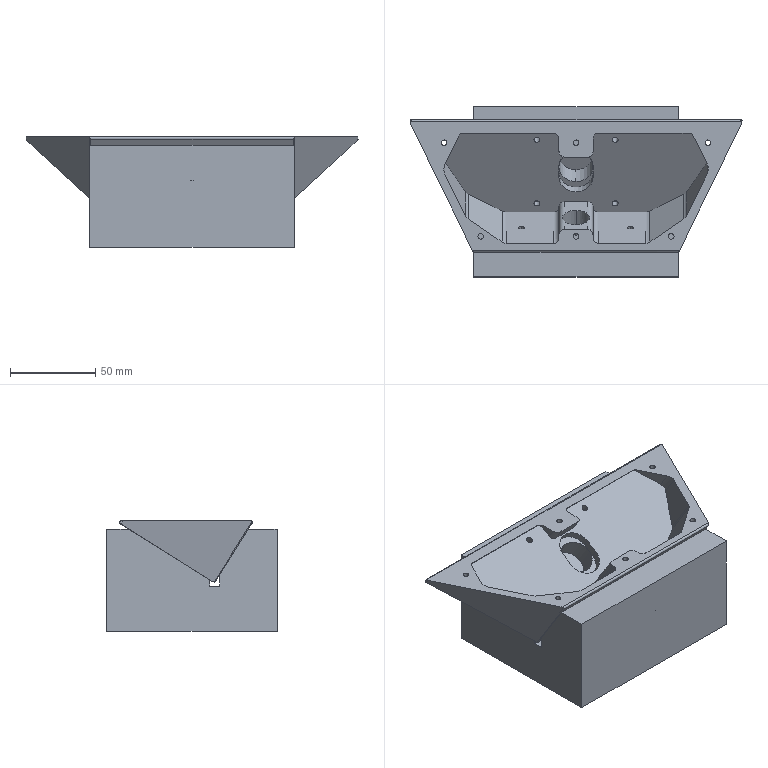NC program | Mastercam | posted with a generic post | part box 195.124 x 100 x 65 mm
Lines 4165 to 4842 of 16336:
N1960 T8 M6
N1970 G0 G90 G17 G57 X-110.144 Y-96.37 A180. S5000 M3
N1980 G43 H8 Z50.
N1990 Z2.
N2000 G1 Z-30.75 F2000.
N2010 X-110.64 Y-95.137 Z-30.87 F4000.
N2020 G3 X-111.435 Y-93.935 Z-31. I-3.34 J-1.343
N2030 G2 X-112.273 Y-92.613 I16.01 J11.086
N2040 X-113.576 Y-88.83 I10.355 J5.683
N2050 X-113.883 Y-85.344 I23.54 J3.826
N2060 X-113.915 Y-81.077 I288.279 J4.267
N2070 X-113.901 Y-78.302 I288.311 J0.
N2080 G1 X-113.898 Y-77.731
N2090 X-113.64 Y-20.441
N2100 X-113.403 Y34.823
N2110 X-113.4 Y84.273
N2120 G2 X-113.401 Y84.454 I13.293 J.181
N2130 X-113.267 Y86.34 I13.294 J0.
N2140 X-111.462 Y90.495 I8.753 J-1.333
N2150 X-108.281 Y93.241 I8.647 J-6.8
N2160 X-105.056 Y94.63 I7.461 J-12.884
N2170 X-101.144 Y95.433 I6.609 J-22.262
N2180 X-95.877 Y95.796 I6.569 J-56.933
N2190 X-86.969 Y95.897 I8.908 J-394.638
N2200 X-85.791 Y95.895 I0. J-394.739
N2210 G1 X-85.208 Y95.896
N2220 X-27.018 Y95.9
N2230 X31.163
N2240 X89.343
N2250 X102.279 Y95.896
N2260 G2 X105.296 Y95.418 I-.106 J-10.441
N2270 X108.627 Y93.428 I-3.009 J-8.816
N2280 X111.314 Y89.692 I-8.103 J-8.664
N2290 X112.58 Y85.789 I-15.667 J-7.237
N2300 X113.189 Y80.814 I-33.929 J-6.676
N2310 X113.376 Y73.478 I-148.458 J-7.468
N2320 X113.395 Y68.203 I-935.543 J-6.004
N2330 G1 X113.396 Y67.62
N2340 X113.4 Y9.431
N2350 Y-48.75
N2360 Y-84.241
N2370 G2 X113.401 Y-84.435 I-13.634 J-.194
N2380 X113.277 Y-86.274 I-13.635 J0.
N2390 X111.503 Y-90.442 I-8.743 J1.26
N2400 X108.331 Y-93.212 I-8.656 J6.71
N2410 X105.1 Y-94.617 I-7.482 J12.788
N2420 X101.182 Y-95.429 I-6.623 J22.106
N2430 X95.91 Y-95.795 I-6.576 J56.467
N2440 X86.999 Y-95.897 I-8.911 J391.025
N2450 X85.822 Y-95.895 I0. J391.127
N2460 G1 X85.238 Y-95.896
N2470 X27.049 Y-95.9
N2480 X-31.132
N2490 X-89.313
N2500 X-102.232 Y-95.897
N2510 G2 X-107.155 Y-94.326 I.188 J9.093
N2520 X-110.442 Y-90.83 I6.221 J9.142
N2530 X-112.018 Y-87.165 I13.024 J7.771
N2540 X-112.848 Y-82.575 I24.925 J6.877
N2550 X-113.124 Y-76.806 I71.423 J6.315
N2560 X-113.155 Y-69.702 I814.918 J7.104
N2570 X-113.135 Y-63.868 I814.949 J0.
N2580 G1 X-113.132 Y-63.286
N2590 X-112.87 Y-5.103
N2600 X-112.704 Y35.018
N2610 X-112.687 Y82.362
N2620 G2 X-109.5 Y89.877 I11.19 J-.312
N2630 X-105.234 Y92.857 I9.984 J-9.751
N2640 X-100.796 Y94.274 I8.212 J-18.06
N2650 X-95.264 Y94.953 I7.658 J-39.495
N2660 X-87.342 Y95.17 I8.137 J-152.602
N2670 X-80.896 Y95.195 I6.996 J-975.226
N2680 G1 X-80.313 Y95.196
N2690 X-22.124 Y95.2
N2700 X36.057
N2710 X94.238
N2720 X99.599 Y95.194
N2730 G2 X107.56 Y91.821 I-.061 J-11.226
N2740 X110.444 Y87.541 I-10.109 J-9.924
N2750 X111.729 Y83.509 I-18.496 J-8.115
N2760 X112.396 Y78.597 I-35.731 J-7.351
N2770 X112.657 Y71.195 I-121.795 J-7.996
N2780 X112.697 Y62.365 I-967.338 J-8.83
N2790 G1 Y61.813
N2800 Y61.23
N2810 X112.7 Y3.044
N2820 Y-55.137
N2830 X112.696 Y-81.997
N2840 Y-82.038
N2850 G2 X109.422 Y-89.958 I-11.218 J0.
N2860 X105.15 Y-92.895 I-9.965 J9.918
N2870 X100.721 Y-94.289 I-8.18 J18.255
N2880 X95.2 Y-94.957 I-7.639 J39.98
N2890 X87.283 Y-95.171 I-8.129 J154.832
N2900 X80.838 Y-95.195 I-6.994 J990.575
N2910 G1 X80.255 Y-95.196
N2920 X22.066 Y-95.2
N2930 X-36.115
N2940 X-94.295
N2950 G2 X-95.459 Y-95.201 I-1.164 J858.632
N2960 X-99.439 Y-95.192 I0. J858.633
N2970 X-107.347 Y-91.783 I.221 J11.391
N2980 X-110.234 Y-87.511 I10.125 J9.954
N2990 X-111.605 Y-83.086 I18.397 J8.125
N3000 X-112.252 Y-77.562 I39.964 J7.481
N3010 X-112.433 Y-70.113 I153.565 J7.449
N3020 X-112.432 Y-69.642 I153.746 J0.
N3030 X-112.435 Y-67.053 I976.965 J2.589
N3040 X-112.428 Y-63.196 I976.968 J0.
N3050 G1 X-112.426 Y-62.613
N3060 X-112.167 Y-4.424
N3070 X-112.007 Y34.536
N3080 X-111.994 Y79.432
N3090 G2 X-111.614 Y82.796 I15.366 J-.035
N3100 X-107.699 Y89.359 I12.416 J-2.956
N3110 X-103.194 Y92.184 I10.539 J-11.805
N3120 X-98.579 Y93.554 I8.897 J-21.507
N3130 X-93.139 Y94.214 I8.032 J-43.464
N3140 X-85.207 Y94.459 I8.497 J-146.591
N3150 X-77. Y94.495 I8.38 J-972.399
N3160 G1 X-76.417 Y94.496
N3170 X-18.229 Y94.5
N3180 X39.952
N3190 X97.12 Y94.491
N3200 G2 X100.557 Y94.049 I-.153 J-14.801
N3210 X107.028 Y90.01 I-3.245 J-12.399
N3220 X109.593 Y85.905 I-12.013 J-10.362
N3230 X111.016 Y81.27 I-20.967 J-8.975
N3240 X111.703 Y75.808 I-42.228 J-8.079
N3250 X111.957 Y67.862 I-141.645 J-8.518
N3260 X111.995 Y59.239 I-971.133 J-8.623
N3270 X111.996 Y59.07 I-971.171 J0.
N3280 G1 Y58.487
N3290 X112. Y.3
N3300 Y-57.881
N3310 X111.992 Y-79.538
N3320 G2 X111.578 Y-82.945 I-15.031 J.101
N3330 X107.591 Y-89.456 I-12.407 J3.12
N3340 X103.493 Y-92.054 I-10.412 J11.892
N3350 X98.849 Y-93.5 I-9.007 J20.745
N3360 X93.377 Y-94.198 I-8.1 J41.734
N3370 X85.425 Y-94.457 I-8.527 J139.687
N3380 X76.801 Y-94.496 I-8.624 J956.163
N3390 G1 X76.632
N3400 X76.049
N3410 X17.862 Y-94.5
N3420 X-40.319
N3430 X-96.941 Y-94.488
N3440 G2 X-100.372 Y-94.027 I.247 J14.859
N3450 X-106.816 Y-89.989 I3.313 J12.447
N3460 X-109.383 Y-85.887 I12.018 J10.375
N3470 X-110.808 Y-81.242 I20.845 J8.937
N3480 X-111.484 Y-75.766 I41.728 J7.934
N3490 X-111.709 Y-67.852 I138.785 J7.914
N3500 X-111.71 Y-67.812 I139.01 J0.
N3510 X-111.72 Y-63.445 I943.857 J4.367
N3520 X-111.709 Y-59.017 I943.867 J0.
N3530 G1 X-111.707 Y-58.435
N3540 X-111.448 Y-.247
N3550 X-111.308 Y34.64
N3560 X-111.29 Y77.225
N3570 G2 X-110.964 Y80.662 I19.033 J-.074
N3580 X-105.882 Y88.956 I13.626 J-2.645
N3590 X-101.909 Y91.299 I10.628 J-13.476
N3600 X-96.649 Y92.842 I9.539 J-22.781
N3610 X-90.639 Y93.525 I8.512 J-48.125
N3620 X-82.156 Y93.762 I9.137 J-175.663
N3630 X-75.124 Y93.793 I7.919 J-979.259
N3640 G1 X-74.541 Y93.794
N3650 X-16.35 Y93.8
N3660 X41.831
N3670 X94.251 Y93.796
N3680 X94.346
N3690 G2 X97.476 Y93.582 I0. J-23.005
N3700 X106.327 Y88.541 I-1.957 J-13.725
N3710 X108.727 Y84.575 I-13.198 J-10.696
N3720 X110.314 Y79.299 I-22.353 J-9.599
N3730 X111.017 Y73.273 I-47.106 J-8.549
N3740 X111.26 Y64.781 I-171.165 J-9.153
N3750 X111.294 Y57.163 I-987.039 J-8.154
N3760 G1 X111.295 Y56.58
N3770 X111.3 Y-1.61
N3780 Y-59.791
N3790 X111.286 Y-77.4
N3800 G2 X110.914 Y-80.902 I-18.234 J.166
N3810 X106.081 Y-88.794 I-13.556 J2.876
N3820 X102.116 Y-91.209 I-10.714 J13.128
N3830 X96.835 Y-92.807 I-9.614 J22.247
N3840 X90.803 Y-93.515 I-8.559 J46.873
N3850 X82.309 Y-93.76 I-9.156 J170.159
N3860 X74.691 Y-93.794 I-8.155 J980.687
N3870 G1 X74.108 Y-93.795
N3880 X15.918 Y-93.8
N3890 X-42.263
N3900 X-94.119 Y-93.794
N3910 X-94.141
N3920 G2 X-97.383 Y-93.556 I0. J22.159
N3930 X-106.18 Y-88.448 I2.103 J13.749
N3940 X-108.554 Y-84.474 I13.317 J10.652
N3950 X-110.115 Y-79.194 I22.463 J9.515
N3960 X-110.793 Y-73.164 I47.16 J8.353
N3970 X-110.999 Y-64.77 I170.528 J8.394
N3980 G1 Y-64.67
N3990 G2 X-111.006 Y-60.93 I978.29 J3.74
N4000 X-110.999 Y-57.052 I978.297 J0.
N4010 G1 X-110.997 Y-56.468
N4020 X-110.739 Y1.721
N4030 X-110.609 Y34.863
N4040 X-110.588 Y75.112
N4050 G2 X-110.308 Y78.659 I24.803 J-.171
N4060 X-104.495 Y88.27 I14.593 J-2.263
N4070 X-99.855 Y90.797 I11.125 J-14.904
N4080 X-94.728 Y92.165 I9.618 J-25.766
N4090 X-88.161 Y92.847 I9.097 J-55.599
N4100 X-79.133 Y93.066 I9.529 J-206.878
N4110 X-73.86 Y93.09 I7.037 J-961.297
N4120 G1 X-73.276 Y93.091
N4130 X-15.081 Y93.1
N4140 X43.1
N4150 X92.026 Y93.095
N4160 X92.103
N4170 G2 X95.789 Y92.865 I0. J-29.661
N4180 X102.272 Y90.377 I-1.973 J-14.827
N4190 X106.615 Y85.767 I-8.836 J-12.674
N4200 X108.718 Y81.155 I-17.073 J-10.572
N4210 X109.932 Y75.456 I-31.105 J-9.607
N4220 X110.443 Y68.451 I-74.269 J-8.933
N4230 X110.589 Y57.784 I-389.902 J-10.667
N4240 X110.588 Y57.188 I-390.048 J0.
N4250 G1 X110.59 Y56.604
N4260 X110.6 Y-1.594
N4270 Y-45.803
N4280 G3 X110.619 Y-46.052 I1.6 J0.
N4290 G2 X110.718 Y-47.313 I-8.001 J-1.261
N4300 X110.704 Y-47.792 I-8.1 J0.
N4310 G3 X110.603 Y-56.28 I357.176 J-8.488
N4320 X110.605 Y-57.469 I357.277 J0.
N4330 G1 X110.604 Y-58.049
N4340 X110.589 Y-75.017
N4350 G2 X110.33 Y-78.525 I-25.607 J.131
N4360 X104.608 Y-88.185 I-14.604 J2.126
N4370 X99.97 Y-90.753 I-11.173 J14.703
N4380 X94.833 Y-92.146 I-9.656 J25.437
N4390 X88.882 Y-92.806 I-8.741 J51.682
N4400 X80.401 Y-93.054 I-9.378 J175.223
N4410 X72.196 Y-93.093 I-8.788 J988.587
N4420 G1 X71.613 Y-93.094
N4430 X13.423 Y-93.1
N4440 X-44.758
N4450 X-91.959 Y-93.093
N4460 X-92.108
N4470 G2 X-95.798 Y-92.826 I0. J25.572
N4480 X-105.74 Y-86.737 I2.149 J14.671
N4490 X-108.033 Y-82.473 I15.2 J10.92
N4500 X-109.424 Y-77.325 I25.264 J9.589
N4510 X-110.069 Y-71.363 I51.092 J8.544
N4520 X-110.285 Y-62.875 I172.118 J8.62
N4530 X-110.295 Y-58.357 I998.404 J4.518
N4540 X-110.286 Y-54.086 I998.414 J0.
N4550 G1 X-110.284 Y-53.503
N4560 X-110.272 Y-50.228
N4570 Y-50.221
N4580 G3 X-110.345 Y-49.742 I-1.6 J0.
N4590 G2 X-110.718 Y-47.313 I7.727 J2.429
N4600 X-110.617 Y-46.038 I8.1 J0.
N4610 G3 X-110.334 Y-42.078 I-42.325 J5.013
N4620 X-110.198 Y-32.387 I-384.119 J10.238
N4630 G1 X-110.195 Y-31.807
N4640 X-109.931 Y26.358
N4650 X-109.9 Y54.843
N4660 X-109.889 Y72.971
N4670 G2 X-109.661 Y76.644 I32.598 J-.178
N4680 X-108.002 Y82.061 I16.294 J-2.028
N4690 X-103.238 Y87.548 I13.99 J-7.335
N4700 X-98.687 Y89.986 I11.398 J-15.815
N4710 X-92.914 Y91.49 I10.304 J-27.707
N4720 X-86.407 Y92.138 I9.263 J-60.01
N4730 X-76.798 Y92.366 I10.148 J-225.103
N4740 X-72.112 Y92.388 I6.994 J-991.545
N4750 G1 X-71.528 Y92.39
N4760 X-13.331 Y92.4
N4770 X44.85
N4780 X90.309 Y92.391
N4790 G2 X93.93 Y92.189 I-.128 J-34.771
N4800 X99.337 Y90.616 I-1.871 J-16.513
N4810 X105.181 Y85.553 I-7.137 J-14.143
N4820 X107.692 Y80.629 I-16.412 J-11.47
N4830 X109.07 Y74.905 I-29.456 J-10.122
N4840 X109.662 Y68.446 I-64.438 J-9.157
N4850 X109.873 Y58.273 I-252.428 J-10.337
N4860 X109.884 Y55.93 I-975.06 J-5.747
N4870 G1 X109.886 Y55.345
N4880 X109.9 Y-2.857
N4890 X109.904 Y-43.436
N4900 G3 X110.038 Y-44.065 I1.6 J.013
N4910 G2 X110.718 Y-47.313 I-7.42 J-3.248
N4920 X110.498 Y-49.19 I-8.1 J0.
N4930 G3 X110.159 Y-51.609 I17.042 J-3.62
N4940 X109.951 Y-56.961 I84.4 J-5.966
N4950 X109.901 Y-66.881 I979.191 J-9.92
N4960 X109.902 Y-68.499 I979.241 J0.
N4970 G1 X109.901 Y-69.08
N4980 G2 X109.904 Y-70.102 I-204.889 J-1.022
N4990 X109.868 Y-73.943 I-204.892 J0.
N5000 X109.447 Y-77.921 I-23.081 J.43
N5010 X103.258 Y-87.534 I-15.216 J2.998
N5020 X98.707 Y-89.978 I-11.406 J15.779
N5030 X92.932 Y-91.487 I-10.31 J27.645
N5040 X86.424 Y-92.137 I-9.267 J59.859
N5050 X76.814 Y-92.366 I-10.15 J224.438
N5060 X72.127 Y-92.388 I-6.994 J988.318
N5070 G1 X71.543 Y-92.39
N5080 X13.346 Y-92.4
N5090 X-44.835
N5100 X-90.317 Y-92.387
N5110 G2 X-94.01 Y-92.146 I.211 J31.66
N5120 X-99.862 Y-90.216 I2.05 J16.051
N5130 X-105.145 Y-85.288 I7.987 J13.857
N5140 X-107.564 Y-80.355 I16.841 J11.322
N5150 X-108.877 Y-74.644 I30.151 J9.939
N5160 X-109.423 Y-68.196 I66.024 J8.837
N5170 X-109.585 Y-59.036 I258.916 J9.16
N5180 X-109.583 Y-58.03 I259.078 J0.
N5190 X-109.584 Y-56.798 I999.64 J1.232
N5200 X-109.583 Y-55.687 I999.641 J0.
N5210 G1 Y-55.102
N5220 G3 X-109.577 Y-54.037 I-96.819 J1.065
N5230 X-109.6 Y-51.939 I-96.825 J0.
N5240 G1 Y-51.898
N5250 G3 X-109.756 Y-51.173 I-1.745 J0.
N5260 G2 X-110.384 Y-49.616 I8.804 J4.451
N5270 G3 X-111.062 Y-48.344 Z-30.928 I-3.451 J-1.024
N5280 G1 X-111.872 Y-47.366 Z-30.865
N5290 G3 X-113.723 Y-46.035 Z-30.75 I-3.47 J-2.872
N5300 X-115.342 Y-45.734 I-1.619 J-4.203 F9500.
N5310 X-119.846 Y-50.238 I0. J-4.504
N5320 X-119.607 Y-51.684 I4.504 J0.
N5330 G1 X-108.76 Y-83.666
N5340 G3 X-95.326 Y-93.494 I13.715 J4.652
N5350 G1 X75.09 Y-96.795
N5360 G3 X76.259 Y-96.806 I1.169 J60.307
N5370 X103.006 Y-90.552 I0. J60.318
N5380 X110.559 Y-81.171 I-6.356 J12.848
N5390 G1 X118.041 Y-51.155
N5400 G3 X118.47 Y-47.625 I-14.298 J3.53
N5410 X118.467 Y-47.295 I-14.727 J0.
N5420 X114.973 Y-43.801 I-3.494 J0.
N5430 X113.316 Y-44.219 I0. J-3.494
N5440 X111.957 Y-45.531 Z-30.845 I1.657 J-3.076 F4000.
N5450 G1 X111.759 Y-45.87 Z-30.865
N5460 X111.118 Y-46.967 Z-30.928
N5470 G3 X110.654 Y-48.332 Z-31. I3.107 J-1.817
N5480 G2 X110.148 Y-50.298 I-8.036 J1.019
N5490 G3 X109.688 Y-52.399 I11.349 J-3.588
N5500 X109.339 Y-56.906 I43.841 J-5.657
N5510 X109.209 Y-65.826 I306.543 J-8.92
N5520 X109.21 Y-66.56 I306.673 J0.
N5530 G1 X109.209 Y-67.139
N5540 G2 X109.21 Y-67.831 I-199.938 J-.692
N5550 X109.152 Y-72.626 I-199.939 J0.
N5560 X108.643 Y-76.934 I-24.188 J.674
N5570 X102.242 Y-86.685 I-15.76 J3.37
N5580 X97.024 Y-89.391 I-11.998 J16.749
N5590 X91.334 Y-90.793 I-10.402 J29.975
N5600 X84.865 Y-91.425 I-9.439 J63.161
N5610 X75.257 Y-91.662 I-10.335 J224.793
N5620 X69.984 Y-91.688 I-7.391 J961.364
N5630 G1 X69.4 Y-91.689
N5640 X11.203 Y-91.7
N5650 X-46.977
N5660 X-88.376 Y-91.687
N5670 G2 X-92.672 Y-91.416 I.047 J34.843
N5680 X-97.486 Y-90.063 I2.284 J17.373
N5690 X-104.052 Y-84.618 I6.752 J14.822
N5700 X-106.714 Y-79.388 I16.859 J11.873
N5710 X-108.079 Y-73.698 I30.219 J10.257
N5720 X-108.678 Y-67.231 I63.598 J9.151
N5730 X-108.87 Y-57.914 I226.012 J9.317
N5740 X-108.869 Y-57.624 I226.204 J0.
N5750 X-108.874 Y-55.871 I902.406 J3.145
N5760 G3 X-108.87 Y-55.345 I-32.379 J.526
N5770 X-108.946 Y-53.127 I-32.383 J0.
N5780 X-109.099 Y-52.56 I-1.595 J-.128
N5790 G2 X-109.974 Y-50.704 I109.099 J52.56
N5800 G3 X-110.827 Y-49.543 Z-30.928 I-3.269 J-1.508
N5810 G1 X-111.769 Y-48.69 Z-30.865
N5820 G3 X-113.801 Y-47.661 Z-30.75 I-2.898 J-3.201
N5830 X-114.667 Y-47.573 I-.866 J-4.23 F9500.
N5840 X-118.985 Y-51.891 I0. J-4.318
N5850 X-118.721 Y-53.377 I4.318 J0.
N5860 G1 X-108.315 Y-81.777
N5870 G3 X-90.706 Y-94.115 I17.662 J6.472
N5880 G1 X86.503 Y-94.617
N5890 X86.579
N5900 G3 X109.028 Y-82.514 I0. J26.872
N5910 X110.11 Y-80.135 I-7.069 J4.651
N5920 G1 X118.414 Y-50.339
N5930 G3 X118.552 Y-49.33 I-3.62 J1.009
N5940 X116.178 Y-45.837 I-3.758 J0.
N5950 X114.867 Y-45.587 I-1.311 J-3.309
N5960 X113.66 Y-45.798 I0. J-3.559
N5970 X112.083 Y-46.928 Z-30.848 I1.207 J-3.348 F4000.
N5980 G1 X111.871 Y-47.194 Z-30.865
N5990 X111.08 Y-48.187 Z-30.928
N6000 G3 X110.425 Y-49.471 Z-31. I2.815 J-2.244
N6010 G2 X109.729 Y-51.232 I-9.276 J2.649
N6020 G3 X109.189 Y-53.22 I9.872 J-3.751
N6030 X108.726 Y-57.554 I34.204 J-5.841
N6040 X108.532 Y-65.368 I173.33 J-8.223
N6050 X108.52 Y-67.102 I929.99 J-7.448
N6060 G2 X108.521 Y-67.431 I-89.043 J-.329
N6070 X108.395 Y-72.162 I-89.044 J0.
N6080 X107.701 Y-76.556 I-22.598 J1.313
N6090 X101.459 Y-85.706 I-16.084 J4.27
N6100 X96.684 Y-88.329 I-12.183 J16.515
N6110 X90.972 Y-89.907 I-10.883 J28.275
N6120 X84.441 Y-90.653 I-9.841 J57.18
N6130 X75.37 Y-90.941 I-10.21 J178.514
N6140 X65.993 Y-90.992 I-9.954 J974.623
N6150 G1 X65.409 Y-90.993
N6160 X7.218 Y-91.
N6170 X-50.963
N6180 X-86.534 Y-90.987
N6190 G2 X-90.654 Y-90.781 I.107 J43.297
N6200 X-95.271 Y-89.744 I1.903 J19.263
N6210 X-103.064 Y-83.848 I5.71 J15.645
N6220 X-105.65 Y-79.06 I16.66 J12.092
N6230 X-107.191 Y-73.345 I28.477 J10.746
N6240 X-107.904 Y-66.815 I57.53 J9.579
N6250 X-108.151 Y-57.763 I181.345 J9.481
N6260 G1 Y-57.644
N6270 G3 X-108.237 Y-54.769 I-47.826 J0.
N6280 G1 Y-54.76
N6290 G3 X-108.422 Y-53.942 I-1.895 J0.
N6300 G2 X-109.439 Y-51.849 I108.422 J53.942
N6310 G3 X-110.304 Y-50.696 Z-30.928 I-3.253 J-1.541
N6320 G1 X-111.598 Y-49.55 Z-30.842
N6330 G3 X-113.196 Y-48.653 Z-30.75 I-2.862 J-3.229
N6340 X-114.46 Y-48.464 I-1.264 J-4.126 F9500.
N6350 X-118.775 Y-52.779 I0. J-4.315
N6360 X-118.446 Y-54.434 I4.315 J0.
N6370 G1 X-107.217 Y-81.469
N6380 G3 X-89.476 Y-93.311 I17.741 J7.368
N6390 X-89.409 Y-93.312 I0. J19.21
N6400 G1 X86.808 Y-92.7
N6410 G3 X106.398 Y-84.378 I-.095 J27.444
N6420 X108.723 Y-80.838 I-8.047 J7.817
N6430 G1 X119.405 Y-54.934
N6440 G3 X119.82 Y-52.838 I-5.082 J2.096
N6450 X114.323 Y-47.341 I-5.497 J0.
N6460 X113.852 Y-47.372 I0. J-3.6
N6470 X111.813 Y-48.361 Z-30.865 I.471 J-3.569 F4000.
N6480 G1 X110.902 Y-49.246 Z-30.928
N6490 G3 X110.091 Y-50.438 Z-31. I2.51 J-2.581
N6500 G2 X109.232 Y-52.284 I-66.541 J29.848
N6510 G3 X108.563 Y-54.604 I9.661 J-4.041
N6520 X108.07 Y-58.945 I34.652 J-6.137
N6530 X107.846 Y-66.178 I149.823 J-8.252
N6540 G2 X107.711 Y-70.583 I-98.785 J.832
N6550 X107.017 Y-75.222 I-25.108 J1.386
N6560 X100.399 Y-84.963 I-16.635 J4.182
N6570 X95.313 Y-87.68 I-12.54 J17.358
N6580 X89.654 Y-89.195 I-10.998 J29.743
N6590 X83.147 Y-89.936 I-10.009 J58.979
N6600 X74.076 Y-90.235 I-10.386 J177.553
N6610 X64.11 Y-90.291 I-10.34 J941.175
N6620 G1 X63.527 Y-90.292
N6630 X5.335 Y-90.3
N6640 X-52.846
N6650 X-84.925 Y-90.286
N6660 G2 X-89.711 Y-90.024 I.12 J46.114
N6670 X-94.684 Y-88.798 I2.149 J19.409
N6680 X-102.271 Y-82.852 I6.366 J15.936
N6690 X-104.971 Y-77.753 I17.383 J12.469
N6700 X-106.464 Y-72.087 I29.755 J10.873
N6710 X-107.178 Y-65.576 I58.911 J9.752
N6720 X-107.427 Y-58.363 I181.424 J9.883
N6730 G3 X-107.562 Y-55.865 I-27.085 J-.212
N6740 X-107.729 Y-55.315 I-1.59 J-.181
N6750 G2 X-108.772 Y-53.235 I107.729 J55.315
N6760 G3 X-109.652 Y-52.093 Z-30.928 I-3.233 J-1.582
N6770 G1 X-111.212 Y-50.744 Z-30.825
N6780 G3 X-112.503 Y-49.969 Z-30.75 I-2.887 J-3.342
N6790 X-114.099 Y-49.67 I-1.596 J-4.117 F9500.
N6800 X-118.515 Y-54.086 I0. J-4.416
N6810 X-118.083 Y-55.99 I4.416 J0.
N6820 G1 X-105.653 Y-81.998
N6830 G3 X-88.458 Y-92.838 I17.195 J8.218
N6840 G1 X-88.343
N6850 X86.078 Y-91.792
N6860 G3 X105.628 Y-83.346 I-.163 J27.226
N6870 X107.415 Y-80.743 I-7.193 J6.853
N6880 G1 X119.173 Y-55.895
N6890 G3 X119.69 Y-53.595 I-4.861 J2.3
N6900 X114.312 Y-48.217 I-5.378 J0.
N6910 X113.338 Y-48.305 I0. J-5.378
N6920 X113.073 Y-48.36 Z-30.763 I.974 J-5.29 F4000.
N6930 X112.142 Y-48.846 Z-30.816 I.492 J-2.08
N6940 G1 X111.662 Y-49.274 Z-30.848
N6950 X110.467 Y-50.34 Z-30.928
N6960 G3 X109.606 Y-51.495 Z-31. I2.397 J-2.686
N6970 G2 X108.575 Y-53.656 I-109.911 J51.125
N6980 G3 X107.891 Y-56.116 I11.101 J-4.409
N6990 X107.393 Y-60.503 I36.793 J-6.404
N7000 X107.152 Y-66.68 I170.39 J-9.732
N7010 G2 X106.815 Y-71.398 I-49.471 J1.157
N7020 X105.602 Y-76.255 I-20.844 J2.628
N7030 X99.527 Y-84.111 I-16.428 J6.426
N7040 X94.486 Y-86.839 I-12.771 J17.579
N7050 X88.839 Y-88.403 I-11.261 J29.681
N7060 X81.693 Y-89.234 I-10.463 J58.847
N7070 X72.041 Y-89.539 I-10.934 J193.463
N7080 X62.665 Y-89.59 I-10.219 J999.503
N7090 G1 X62.082 Y-89.592
N7100 X3.889 Y-89.6
N7110 X-54.292
N7120 X-82.858 Y-89.59
N7130 G2 X-87.444 Y-89.415 I.089 J62.785
N7140 X-92.161 Y-88.556 I1.827 J23.409
N7150 X-101.343 Y-82.077 I4.983 J16.807
N7160 X-104.087 Y-77.027 I17.41 J12.733
N7170 X-105.651 Y-71.369 I29.386 J11.165
N7180 X-106.424 Y-64.837 I56.832 J10.039
N7190 X-106.704 Y-58.914 I194.477 J12.172
N7200 G3 X-106.838 Y-57.247 I-20.355 J-.789
N7210 X-107.013 Y-56.688 I-1.588 J-.19
N7220 G2 X-108.082 Y-54.621 I107.013 J56.688
N7230 G3 X-108.976 Y-53.491 Z-30.928 I-3.213 J-1.624
N7240 G1 X-110.576 Y-52.145 Z-30.824
N7250 G3 X-111.859 Y-51.414 Z-30.75 I-2.618 J-3.11
N7260 X-113.194 Y-51.189 I-1.335 J-3.841 F9500.
N7270 X-117.26 Y-55.255 I0. J-4.066
N7280 X-116.821 Y-57.094 I4.066 J0.
N7290 G1 X-103.744 Y-82.884
N7300 G3 X-87.579 Y-92.812 I16.165 J8.196
N7310 G1 X-87.544
N7320 X84.208 Y-92.481
N7330 G3 X107.762 Y-77.23 I-.05 J25.892
N7340 G1 X117.835 Y-54.883
N7350 G3 X118.194 Y-53.215 I-3.701 J1.668
N7360 X114.134 Y-49.155 I-4.06 J0.
N7370 X112.791 Y-49.384 I0. J-4.06
N7380 X111.463 Y-50.157 Z-30.827 I1.343 J-3.831 F4000.
N7390 G1 X111.409 Y-50.205 Z-30.83
N7400 X109.935 Y-51.493 Z-30.928
N7410 G3 X109.061 Y-52.639 Z-31. I2.368 J-2.711
N7420 G2 X108.05 Y-54.685 I-109.061 J52.639
N7430 G3 X107.328 Y-56.999 I9.625 J-4.274
N7440 X106.762 Y-61.289 I32.504 J-6.469
N7450 X106.476 Y-66.361 I187.201 J-13.099
N7460 G2 X105.981 Y-71.183 I-42.427 J1.917
N7470 X104.356 Y-76.426 I-19.835 J3.276
N7480 X99.326 Y-82.768 I-16.298 J7.76
N7490 X93.644 Y-86.019 I-13.512 J17.025
N7500 X87.336 Y-87.745 I-11.678 J30.28
N7510 X80.234 Y-88.536 I-10.546 J62.439
N7520 X70.594 Y-88.836 I-11.057 J200.229
N7530 X61.218 Y-88.89 I-10.345 J991.635
N7540 G1 X60.635 Y-88.891
N7550 X2.442 Y-88.9
N7560 X-55.739
N7570 X-81.399 Y-88.888
N7580 X-81.477
N7590 G2 X-86.647 Y-88.664 I0. J59.71
N7600 X-91.347 Y-87.743 I2.151 J23.445
N7610 X-100.154 Y-81.669 I5.264 J17.053
N7620 X-103.352 Y-75.956 I17.205 J13.382
N7630 X-105.025 Y-69.65 I30.621 J11.499
N7640 X-105.736 Y-63.204 I63.182 J10.237
N7650 G3 X-105.998 Y-59.343 I-215.809 J-12.659
N7660 X-106.084 Y-58.629 I-13.714 J-1.292
N7670 X-106.265 Y-58.077 I-1.585 J-.215
N7680 G2 X-107.362 Y-56.024 I106.265 J58.077
N7690 G3 X-108.271 Y-54.906 Z-30.928 I-3.191 J-1.665
N7700 G1 X-109.887 Y-53.58 Z-30.824
N7710 G3 X-111.174 Y-52.854 Z-30.75 I-2.717 J-3.314
N7720 X-112.604 Y-52.608 I-1.43 J-4.04 F9500.
N7730 X-116.89 Y-56.894 I0. J-4.286
N7740 X-116.302 Y-59.059 I4.286 J0.
N7750 G1 X-103.101 Y-81.602
N7760 G3 X-84.996 Y-91.98 I18.105 J10.603
N7770 G1 X-84.827
N7780 X83.667 Y-90.63
N7790 G3 X109.197 Y-73.611 I-.225 J27.995
N7800 G1 X116.924 Y-55.481
N7810 G3 X117.22 Y-54.034 I-3.394 J1.447
N7820 X113.53 Y-50.344 I-3.69 J0.
N7830 X112.157 Y-50.609 I0. J-3.69
N7840 X111.135 Y-51.227 Z-30.81 I1.373 J-3.425 F4000.
N7850 G1 X110.918 Y-51.412 Z-30.824
N7860 X109.328 Y-52.769 Z-30.928
N7870 G3 X108.441 Y-53.905 Z-31. I2.337 J-2.739
N7880 G2 X107.361 Y-56.045 I-108.749 J53.536
N7890 G3 X106.634 Y-58.47 I10.762 J-4.55
N7900 X106.06 Y-62.85 I36.307 J-6.983
N7910 X105.836 Y-65.724 I258.984 J-21.653
N7920 G2 X105.226 Y-70.517 I-42.812 J3.012
N7930 X103.324 Y-76.061 I-20.136 J3.808
N7940 X97.861 Y-82.422 I-16.559 J8.696
N7950 X92.186 Y-85.45 I-13.564 J18.586
N7960 X85.937 Y-87.074 I-11.699 J32.184
N7970 X78.871 Y-87.835 I-10.637 J65.562
N7980 X68.65 Y-88.14 I-11.401 J210.578
N7990 X60.447 Y-88.187 I-9.797 J990.888
N8000 G1 X59.863 Y-88.189
N8010 X1.667 Y-88.2
N8020 X-56.514
N8030 X-79.843 Y-88.188
N8040 X-79.856
N8050 G2 X-85.009 Y-87.995 I0. J68.914
N8060 X-89.581 Y-87.222 I2.057 J26.079
N8070 X-99.415 Y-80.7 I4.638 J17.668
N8080 X-102.576 Y-75.022 I17.635 J13.537
N8090 X-104.265 Y-68.737 I30.945 J11.682
N8100 X-104.969 Y-62.994 I65.647 J10.963
N8110 G3 X-105.289 Y-60.021 I-42.522 J-3.086
N8120 X-105.473 Y-59.503 I-1.578 J-.268
N8130 G2 X-106.597 Y-57.465 I105.473 J59.503
N8140 G3 X-107.521 Y-56.359 Z-30.928 I-3.169 J-1.708
N8150 G1 X-109.156 Y-55.055 Z-30.824
N8160 G3 X-110.451 Y-54.345 Z-30.75 I-2.698 J-3.384
N8170 X-111.854 Y-54.111 I-1.403 J-4.094 F9500.
N8180 X-116.182 Y-58.439 I0. J-4.328
N8190 X-115.466 Y-60.821 I4.328 J0.
N8200 G1 X-101.789 Y-81.557
N8210 G3 X-86.556 Y-89.757 I15.233 J10.049
N8220 G1 X-86.547
N8230 X83.109 Y-89.672
N8240 G3 X105.864 Y-76.3 I-.013 J26.069
N8250 G1 X116.42 Y-57.371
N8260 G3 X116.915 Y-55.467 I-3.414 J1.904
N8270 X113.006 Y-51.558 I-3.909 J0.
N8280 X111.635 Y-51.806 I0. J-3.909
N8290 X110.5 Y-52.466 Z-30.816 I1.371 J-3.661 F4000.
N8300 G1 X110.373 Y-52.572 Z-30.824
N8310 X108.768 Y-53.913 Z-30.928
N8320 G3 X107.87 Y-55.039 Z-31. I2.308 J-2.763
N8330 G2 X106.83 Y-57.031 I-107.87 J55.039
N8340 G3 X106.068 Y-59.296 I9.176 J-4.349
N8350 X105.455 Y-63.116 I33.634 J-7.358
N8360 X105.196 Y-65.417 I319.811 J-37.075
N8370 G2 X104.408 Y-70.22 I-41.29 J4.315
N8380 X102.32 Y-75.648 I-20.506 J4.771
N8390 X96.799 Y-81.777 I-16.749 J9.536
N8400 X91.146 Y-84.732 I-13.682 J19.287
N8410 X84.925 Y-86.342 I-11.837 J32.917
N8420 X77.865 Y-87.115 I-10.793 J65.979
N8430 X67.639 Y-87.434 I-11.544 J205.822
N8440 X58.848 Y-87.487 I-10.154 J957.04
N8450 G1 X58.265 Y-87.488
N8460 X.069 Y-87.5
N8470 X-58.112
N8480 X-78.536 Y-87.486
N8490 G2 X-83.663 Y-87.301 I.092 J73.579
N8500 X-88.954 Y-86.381 I1.975 J27.051
N8510 X-99.141 Y-79.122 I5.11 J17.95
N8520 X-102.051 Y-73.447 I19.335 J13.497
N8530 X-103.614 Y-67.24 I33.558 J11.748
N8540 X-104.204 Y-62.966 I99.407 J15.906
N8550 G3 X-104.427 Y-61.504 I-22.032 J-2.61
N8560 X-104.616 Y-60.997 I-1.571 J-.299
N8570 G2 X-105.769 Y-58.975 I104.616 J60.997
N8580 G3 X-106.709 Y-57.883 Z-30.928 I-3.144 J-1.754
N8590 G1 X-108.361 Y-56.602 Z-30.824
N8600 G3 X-109.666 Y-55.907 Z-30.75 I-2.684 J-3.465
N8610 X-111.045 Y-55.684 I-1.379 J-4.16 F9500.
N8620 X-115.428 Y-60.067 I0. J-4.383
N8630 X-114.542 Y-62.709 I4.383 J0.
N8640 G1 X-99.841 Y-82.169
N8650 G3 X-83.341 Y-90.383 I16.5 J12.465
N8660 X-83.163 Y-90.382 I0. J20.679
N8670 G1 X77.515 Y-88.998
N8680 G3 X88.54 Y-87.885 I-.519 J60.286
N8690 X105.295 Y-74.745 I-4.48 J22.967
N8700 G1 X114.141 Y-55.63
N8710 G3 X114.344 Y-54.709 I-1.991 J.921
N8720 X112.15 Y-52.515 I-2.194 J0.
N8730 X110.926 Y-52.889 I0. J-2.194